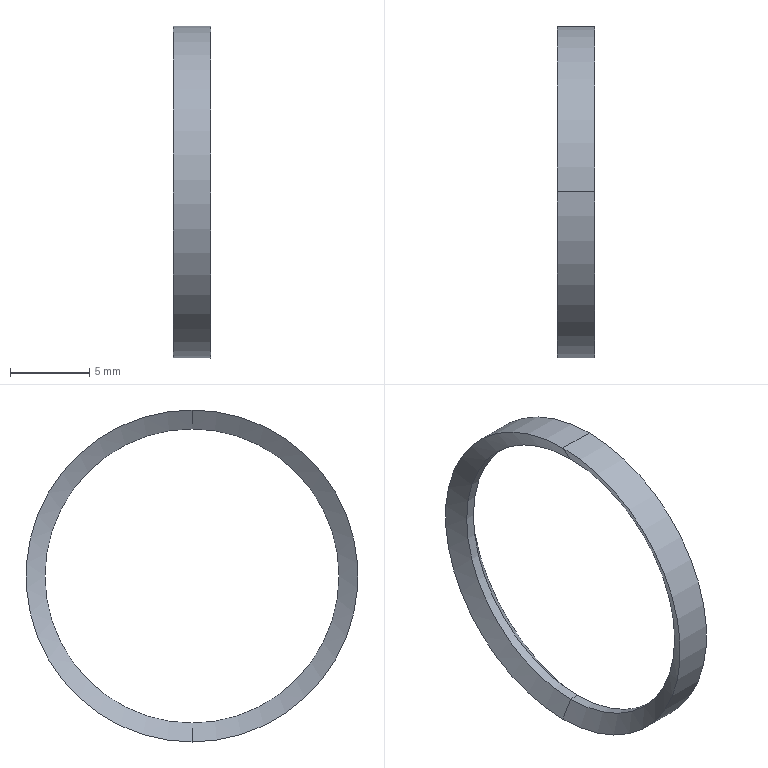Part | STEP file | 2026.6.15-Main Assembly图.sldasm-Part-219 | 1 solid | 9 faces | box 2.343 x 21 x 21 mm | volume 106.322 mm3 | cylinder 4 | cone 4 | plane 1 | commonest cylinder face diameters 18.6 x2 21 x2
STEP:
#1=CARTESIAN_POINT('',(-1618.788,1424.264,3398.636));
#2=VERTEX_POINT('',#1);
#3=CARTESIAN_POINT('',(-1618.788,1424.264,3417.536));
#4=VERTEX_POINT('',#3);
#5=CARTESIAN_POINT('',(-1618.788,1424.264,3408.086));
#6=DIRECTION('',(1.,0.,0.));
#7=DIRECTION('',(0.,0.,-1.));
#8=AXIS2_PLACEMENT_3D('',#5,#6,#7);
#9=CIRCLE('',#8,9.45);
#10=EDGE_CURVE('',#2,#4,#9,.T.);
#11=ORIENTED_EDGE('',*,*,#10,.T.);
#12=CARTESIAN_POINT('',(-1618.788,1424.264,3408.086));
#13=DIRECTION('',(1.,0.,0.));
#14=DIRECTION('',(0.,0.,-1.));
#15=AXIS2_PLACEMENT_3D('',#12,#13,#14);
#16=CIRCLE('',#15,9.45);
#17=EDGE_CURVE('',#4,#2,#16,.T.);
#18=ORIENTED_EDGE('',*,*,#17,.T.);
#19=EDGE_LOOP('',(#11,#18));
#20=FACE_OUTER_BOUND('',#19,.T.);
#21=CARTESIAN_POINT('',(-1618.788,1424.264,3417.386));
#22=VERTEX_POINT('',#21);
#23=CARTESIAN_POINT('',(-1618.788,1424.264,3398.786));
#24=VERTEX_POINT('',#23);
#25=CARTESIAN_POINT('',(-1618.788,1424.264,3408.086));
#26=DIRECTION('',(-1.,0.,0.));
#27=DIRECTION('',(0.,0.,1.));
#28=AXIS2_PLACEMENT_3D('',#25,#26,#27);
#29=CIRCLE('',#28,9.3);
#30=EDGE_CURVE('',#22,#24,#29,.T.);
#31=ORIENTED_EDGE('',*,*,#30,.T.);
#32=CARTESIAN_POINT('',(-1618.788,1424.264,3408.086));
#33=DIRECTION('',(-1.,0.,0.));
#34=DIRECTION('',(0.,0.,1.));
#35=AXIS2_PLACEMENT_3D('',#32,#33,#34);
#36=CIRCLE('',#35,9.3);
#37=EDGE_CURVE('',#24,#22,#36,.T.);
#38=ORIENTED_EDGE('',*,*,#37,.T.);
#39=EDGE_LOOP('',(#31,#38));
#40=FACE_BOUND('',#39,.T.);
#41=CARTESIAN_POINT('',(-1618.788,1424.264,3408.086));
#42=DIRECTION('',(-1.,0.,0.));
#43=DIRECTION('',(0.,0.,1.));
#44=AXIS2_PLACEMENT_3D('',#41,#42,#43);
#45=PLANE('',#44);
#46=ADVANCED_FACE('',(#20,#40),#45,.F.);
#47=CARTESIAN_POINT('',(-1619.388,1424.264,3398.786));
#48=VERTEX_POINT('',#47);
#49=CARTESIAN_POINT('',(-1619.388,1424.264,3398.786));
#50=DIRECTION('',(1.,0.,0.));
#51=VECTOR('',#50,1000.);
#52=LINE('',#49,#51);
#53=EDGE_CURVE('',#48,#24,#52,.T.);
#54=ORIENTED_EDGE('',*,*,#53,.T.);
#55=ORIENTED_EDGE('',*,*,#30,.F.);
#56=CARTESIAN_POINT('',(-1619.388,1424.264,3417.386));
#57=VERTEX_POINT('',#56);
#58=CARTESIAN_POINT('',(-1619.388,1424.264,3417.386));
#59=DIRECTION('',(1.,0.,0.));
#60=VECTOR('',#59,1000.);
#61=LINE('',#58,#60);
#62=EDGE_CURVE('',#57,#22,#61,.T.);
#63=ORIENTED_EDGE('',*,*,#62,.F.);
#64=CARTESIAN_POINT('',(-1619.388,1424.264,3408.086));
#65=DIRECTION('',(-1.,0.,0.));
#66=DIRECTION('',(0.,0.,1.));
#67=AXIS2_PLACEMENT_3D('',#64,#65,#66);
#68=CIRCLE('',#67,9.3);
#69=EDGE_CURVE('',#57,#48,#68,.T.);
#70=ORIENTED_EDGE('',*,*,#69,.T.);
#71=EDGE_LOOP('',(#54,#55,#63,#70));
#72=FACE_OUTER_BOUND('',#71,.T.);
#73=CARTESIAN_POINT('',(-1619.388,1424.264,3408.086));
#74=DIRECTION('',(-1.,0.,0.));
#75=DIRECTION('',(0.,0.,-1.));
#76=AXIS2_PLACEMENT_3D('',#73,#74,#75);
#77=CYLINDRICAL_SURFACE('',#76,9.3);
#78=ADVANCED_FACE('',(#72),#77,.F.);
#79=CARTESIAN_POINT('',(-1617.738,1424.264,3418.586));
#80=VERTEX_POINT('',#79);
#81=CARTESIAN_POINT('',(-1617.738,1424.264,3418.586));
#82=DIRECTION('',(0.7071,0.,0.7071));
#83=VECTOR('',#82,1000.);
#84=LINE('',#81,#83);
#85=EDGE_CURVE('',#4,#80,#84,.T.);
#86=ORIENTED_EDGE('',*,*,#85,.F.);
#87=ORIENTED_EDGE('',*,*,#10,.F.);
#88=CARTESIAN_POINT('',(-1617.738,1424.264,3397.586));
#89=VERTEX_POINT('',#88);
#90=CARTESIAN_POINT('',(-1617.738,1424.264,3397.586));
#91=DIRECTION('',(0.7071,0.,-0.7071));
#92=VECTOR('',#91,1000.);
#93=LINE('',#90,#92);
#94=EDGE_CURVE('',#2,#89,#93,.T.);
#95=ORIENTED_EDGE('',*,*,#94,.T.);
#96=CARTESIAN_POINT('',(-1617.738,1424.264,3408.086));
#97=DIRECTION('',(-1.,0.,0.));
#98=DIRECTION('',(0.,0.,1.));
#99=AXIS2_PLACEMENT_3D('',#96,#97,#98);
#100=CIRCLE('',#99,10.5);
#101=EDGE_CURVE('',#80,#89,#100,.T.);
#102=ORIENTED_EDGE('',*,*,#101,.F.);
#103=EDGE_LOOP('',(#86,#87,#95,#102));
#104=FACE_OUTER_BOUND('',#103,.T.);
#105=CARTESIAN_POINT('',(-1617.738,1424.264,3408.086));
#106=DIRECTION('',(1.,0.,0.));
#107=DIRECTION('',(0.,0.,1.));
#108=AXIS2_PLACEMENT_3D('',#105,#106,#107);
#109=CONICAL_SURFACE('',#108,10.5,0.7854);
#110=ADVANCED_FACE('',(#104),#109,.F.);
#111=CARTESIAN_POINT('',(-1620.081,1424.264,3397.586));
#112=VERTEX_POINT('',#111);
#113=CARTESIAN_POINT('',(-1620.081,1424.264,3397.586));
#114=DIRECTION('',(0.5,0.,0.866));
#115=VECTOR('',#114,1000.);
#116=LINE('',#113,#115);
#117=EDGE_CURVE('',#112,#48,#116,.T.);
#118=ORIENTED_EDGE('',*,*,#117,.T.);
#119=ORIENTED_EDGE('',*,*,#69,.F.);
#120=CARTESIAN_POINT('',(-1620.081,1424.264,3418.586));
#121=VERTEX_POINT('',#120);
#122=CARTESIAN_POINT('',(-1620.081,1424.264,3418.586));
#123=DIRECTION('',(0.5,0.,-0.866));
#124=VECTOR('',#123,1000.);
#125=LINE('',#122,#124);
#126=EDGE_CURVE('',#121,#57,#125,.T.);
#127=ORIENTED_EDGE('',*,*,#126,.F.);
#128=CARTESIAN_POINT('',(-1620.081,1424.264,3408.086));
#129=DIRECTION('',(1.,0.,0.));
#130=DIRECTION('',(0.,0.,1.));
#131=AXIS2_PLACEMENT_3D('',#128,#129,#130);
#132=CIRCLE('',#131,10.5);
#133=EDGE_CURVE('',#112,#121,#132,.T.);
#134=ORIENTED_EDGE('',*,*,#133,.F.);
#135=EDGE_LOOP('',(#118,#119,#127,#134));
#136=FACE_OUTER_BOUND('',#135,.T.);
#137=CARTESIAN_POINT('',(-1620.081,1424.264,3408.086));
#138=DIRECTION('',(-1.,0.,0.));
#139=DIRECTION('',(0.,0.,-1.));
#140=AXIS2_PLACEMENT_3D('',#137,#138,#139);
#141=CONICAL_SURFACE('',#140,10.5,1.047);
#142=ADVANCED_FACE('',(#136),#141,.F.);
#143=CARTESIAN_POINT('',(-1621.788,1424.264,3397.586));
#144=DIRECTION('',(1.,0.,0.));
#145=VECTOR('',#144,1000.);
#146=LINE('',#143,#145);
#147=EDGE_CURVE('',#112,#89,#146,.T.);
#148=ORIENTED_EDGE('',*,*,#147,.T.);
#149=CARTESIAN_POINT('',(-1617.738,1424.264,3408.086));
#150=DIRECTION('',(-1.,0.,0.));
#151=DIRECTION('',(0.,0.,1.));
#152=AXIS2_PLACEMENT_3D('',#149,#150,#151);
#153=CIRCLE('',#152,10.5);
#154=EDGE_CURVE('',#89,#80,#153,.T.);
#155=ORIENTED_EDGE('',*,*,#154,.T.);
#156=CARTESIAN_POINT('',(-1621.788,1424.264,3418.586));
#157=DIRECTION('',(1.,0.,0.));
#158=VECTOR('',#157,1000.);
#159=LINE('',#156,#158);
#160=EDGE_CURVE('',#121,#80,#159,.T.);
#161=ORIENTED_EDGE('',*,*,#160,.F.);
#162=CARTESIAN_POINT('',(-1620.081,1424.264,3408.086));
#163=DIRECTION('',(1.,0.,0.));
#164=DIRECTION('',(0.,0.,1.));
#165=AXIS2_PLACEMENT_3D('',#162,#163,#164);
#166=CIRCLE('',#165,10.5);
#167=EDGE_CURVE('',#121,#112,#166,.T.);
#168=ORIENTED_EDGE('',*,*,#167,.T.);
#169=EDGE_LOOP('',(#148,#155,#161,#168));
#170=FACE_OUTER_BOUND('',#169,.T.);
#171=CARTESIAN_POINT('',(-1621.788,1424.264,3408.086));
#172=DIRECTION('',(-1.,0.,0.));
#173=DIRECTION('',(0.,0.,-1.));
#174=AXIS2_PLACEMENT_3D('',#171,#172,#173);
#175=CYLINDRICAL_SURFACE('',#174,10.5);
#176=ADVANCED_FACE('',(#170),#175,.T.);
#177=ORIENTED_EDGE('',*,*,#37,.F.);
#178=ORIENTED_EDGE('',*,*,#53,.F.);
#179=CARTESIAN_POINT('',(-1619.388,1424.264,3408.086));
#180=DIRECTION('',(-1.,0.,0.));
#181=DIRECTION('',(0.,0.,1.));
#182=AXIS2_PLACEMENT_3D('',#179,#180,#181);
#183=CIRCLE('',#182,9.3);
#184=EDGE_CURVE('',#48,#57,#183,.T.);
#185=ORIENTED_EDGE('',*,*,#184,.T.);
#186=ORIENTED_EDGE('',*,*,#62,.T.);
#187=EDGE_LOOP('',(#177,#178,#185,#186));
#188=FACE_OUTER_BOUND('',#187,.T.);
#189=CARTESIAN_POINT('',(-1619.388,1424.264,3408.086));
#190=DIRECTION('',(-1.,0.,0.));
#191=DIRECTION('',(0.,0.,-1.));
#192=AXIS2_PLACEMENT_3D('',#189,#190,#191);
#193=CYLINDRICAL_SURFACE('',#192,9.3);
#194=ADVANCED_FACE('',(#188),#193,.F.);
#195=ORIENTED_EDGE('',*,*,#17,.F.);
#196=ORIENTED_EDGE('',*,*,#85,.T.);
#197=ORIENTED_EDGE('',*,*,#154,.F.);
#198=ORIENTED_EDGE('',*,*,#94,.F.);
#199=EDGE_LOOP('',(#195,#196,#197,#198));
#200=FACE_OUTER_BOUND('',#199,.T.);
#201=CARTESIAN_POINT('',(-1617.738,1424.264,3408.086));
#202=DIRECTION('',(1.,0.,0.));
#203=DIRECTION('',(0.,0.,1.));
#204=AXIS2_PLACEMENT_3D('',#201,#202,#203);
#205=CONICAL_SURFACE('',#204,10.5,0.7854);
#206=ADVANCED_FACE('',(#200),#205,.F.);
#207=ORIENTED_EDGE('',*,*,#184,.F.);
#208=ORIENTED_EDGE('',*,*,#117,.F.);
#209=ORIENTED_EDGE('',*,*,#167,.F.);
#210=ORIENTED_EDGE('',*,*,#126,.T.);
#211=EDGE_LOOP('',(#207,#208,#209,#210));
#212=FACE_OUTER_BOUND('',#211,.T.);
#213=CARTESIAN_POINT('',(-1620.081,1424.264,3408.086));
#214=DIRECTION('',(-1.,0.,0.));
#215=DIRECTION('',(0.,0.,-1.));
#216=AXIS2_PLACEMENT_3D('',#213,#214,#215);
#217=CONICAL_SURFACE('',#216,10.5,1.047);
#218=ADVANCED_FACE('',(#212),#217,.F.);
#219=ORIENTED_EDGE('',*,*,#101,.T.);
#220=ORIENTED_EDGE('',*,*,#147,.F.);
#221=ORIENTED_EDGE('',*,*,#133,.T.);
#222=ORIENTED_EDGE('',*,*,#160,.T.);
#223=EDGE_LOOP('',(#219,#220,#221,#222));
#224=FACE_OUTER_BOUND('',#223,.T.);
#225=CARTESIAN_POINT('',(-1621.788,1424.264,3408.086));
#226=DIRECTION('',(-1.,0.,0.));
#227=DIRECTION('',(0.,0.,-1.));
#228=AXIS2_PLACEMENT_3D('',#225,#226,#227);
#229=CYLINDRICAL_SURFACE('',#228,10.5);
#230=ADVANCED_FACE('',(#224),#229,.T.);
#231=CLOSED_SHELL('',(#46,#78,#110,#142,#176,#194,#206,#218,#230));
#232=MANIFOLD_SOLID_BREP('',#231);
#233=CARTESIAN_POINT('',(0.,0.,0.));
#234=DIRECTION('',(0.,0.,1.));
#235=DIRECTION('',(1.,0.,0.));
#236=AXIS2_PLACEMENT_3D('',#233,#234,#235);
#237=(LENGTH_UNIT()NAMED_UNIT(*)SI_UNIT(.MILLI.,.METRE.));
#238=UNCERTAINTY_MEASURE_WITH_UNIT(LENGTH_MEASURE(0.00001),#237,'','');
#239=(NAMED_UNIT(*)PLANE_ANGLE_UNIT()SI_UNIT($,.RADIAN.));
#240=(NAMED_UNIT(*)SI_UNIT($,.STERADIAN.)SOLID_ANGLE_UNIT());
#241=(GEOMETRIC_REPRESENTATION_CONTEXT(3)GLOBAL_UNCERTAINTY_ASSIGNED_CONTEXT((#238))GLOBAL_UNIT_ASSIGNED_CONTEXT((#237,#239,#240))REPRESENTATION_CONTEXT('',''));
#242=ADVANCED_BREP_SHAPE_REPRESENTATION('',(#232,#236),#241);